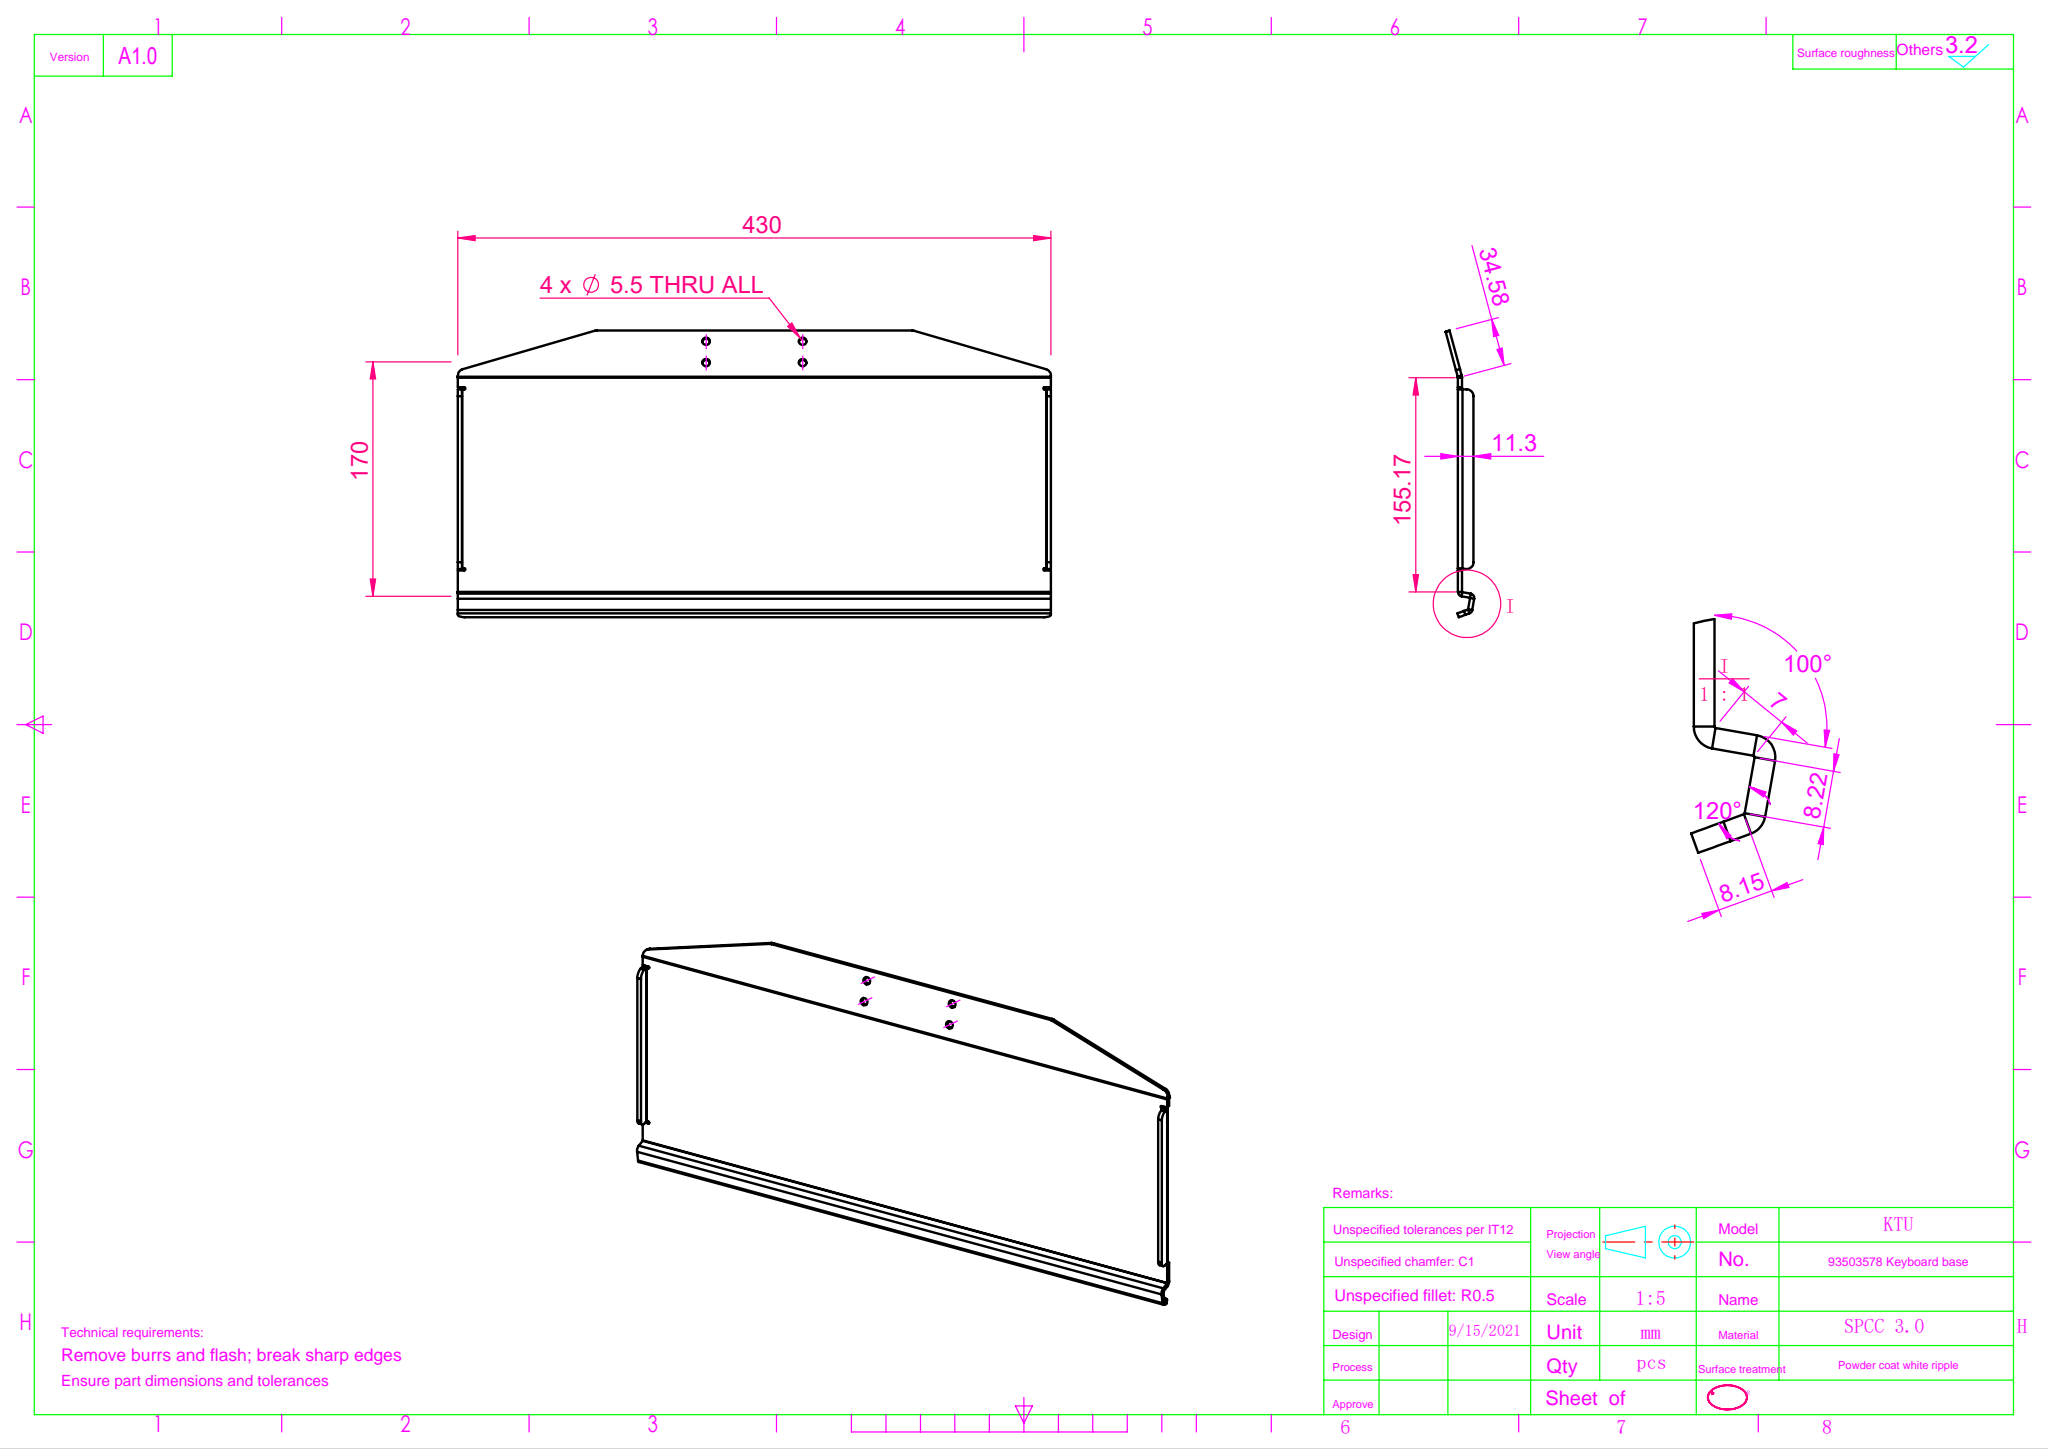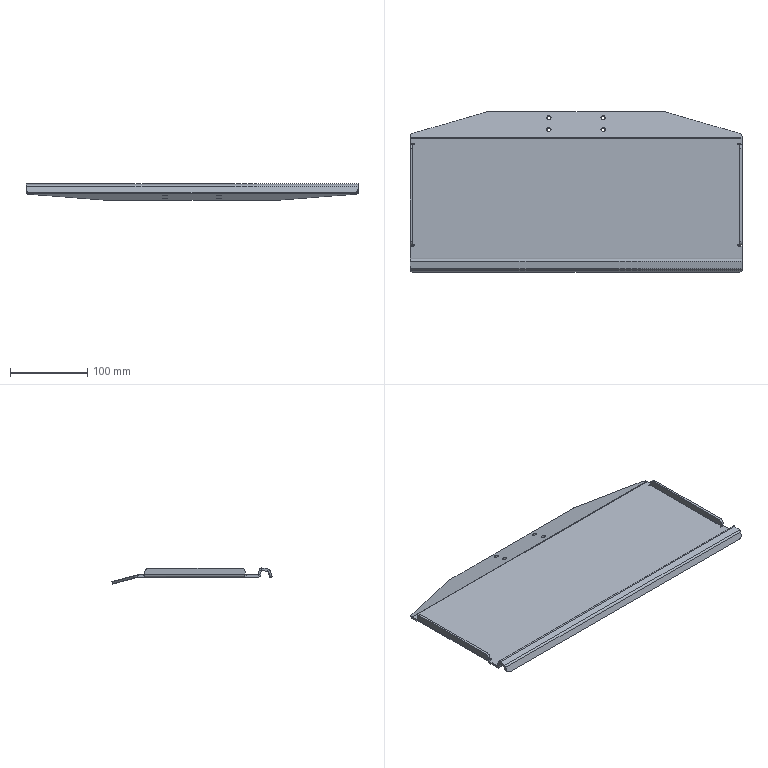Part | SolidWorks | features EdgeFlange 5, Fillet 2, Chamfer 1, FlatPattern 1, HoleWzd 1, SMBaseFlange 1, SheetMetal 1 | 1 solid | 90 faces | box 430 x 207.698 x 20.788 mm | volume 279577 mm3 | plane 54 | cylinder 34 | spline 2 | commonest cylinder face diameters 10 x10 5.5 x8 0.4 x6 6.4 x6 1.5 x4